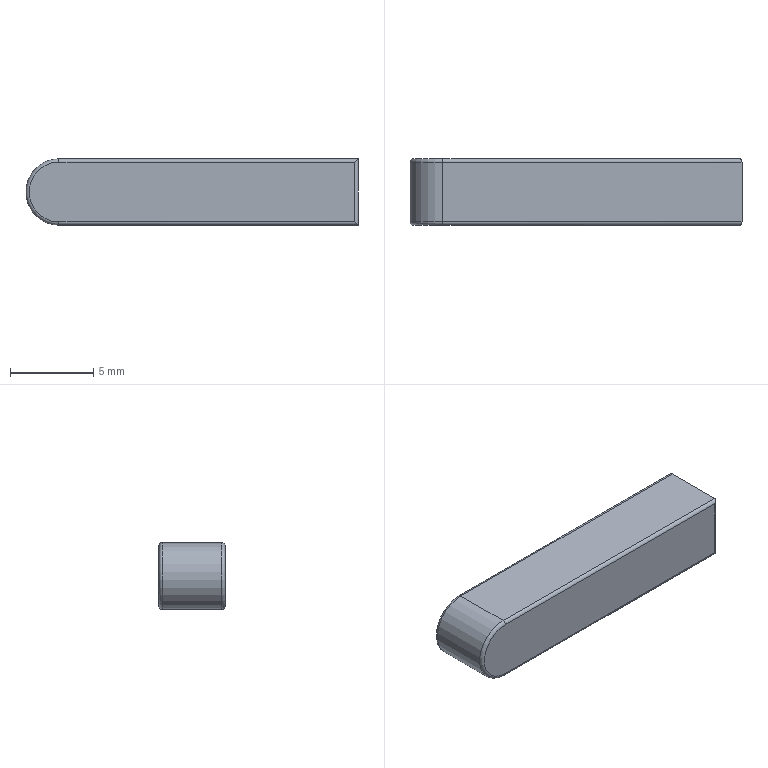Part | STEP file | 1 solid | 14 faces | box 20 x 4 x 4 mm | volume 312.344 mm3 | cylinder 7 | plane 5 | torus 2 | commonest cylinder face diameters 0.4 x6 4 x1
STEP:
#1=CARTESIAN_POINT('',(0.,0.,0.));
#2=DIRECTION('',(0.,0.,1.));
#3=DIRECTION('',(1.,0.,0.));
#4=AXIS2_PLACEMENT_3D('',#1,#2,#3);
#5=CARTESIAN_POINT('',(0.,1.8,-2.));
#6=VERTEX_POINT('',#5);
#7=CARTESIAN_POINT('',(0.,-1.8,-2.));
#8=VERTEX_POINT('',#7);
#9=CARTESIAN_POINT('',(0.,2.,-2.));
#10=DIRECTION('',(0.,-1.,0.));
#11=VECTOR('',#10,1.);
#12=LINE('',#9,#11);
#13=CARTESIAN_POINT('',(0.,2.,0.));
#14=DIRECTION('',(0.,-1.,0.));
#15=DIRECTION('',(0.,0.,-1.));
#16=AXIS2_PLACEMENT_3D('',#13,#14,#15);
#17=CYLINDRICAL_SURFACE('',#16,2.);
#18=CARTESIAN_POINT('',(6.283,0.));
#19=DIRECTION('',(0.,1.));
#20=VECTOR('',#19,1.);
#21=LINE('',#18,#20);
#22=(GEOMETRIC_REPRESENTATION_CONTEXT(2)PARAMETRIC_REPRESENTATION_CONTEXT()REPRESENTATION_CONTEXT('',''));
#23=DEFINITIONAL_REPRESENTATION('',(#21),#22);
#24=PCURVE('',#17,#23);
#25=CARTESIAN_POINT('',(0.,2.,-2.));
#26=DIRECTION('',(0.,0.,1.));
#27=DIRECTION('',(1.,0.,0.));
#28=AXIS2_PLACEMENT_3D('',#25,#26,#27);
#29=PLANE('',#28);
#30=CARTESIAN_POINT('',(0.,0.));
#31=DIRECTION('',(0.,-1.));
#32=VECTOR('',#31,1.);
#33=LINE('',#30,#32);
#34=(GEOMETRIC_REPRESENTATION_CONTEXT(2)PARAMETRIC_REPRESENTATION_CONTEXT()REPRESENTATION_CONTEXT('',''));
#35=DEFINITIONAL_REPRESENTATION('',(#33),#34);
#36=PCURVE('',#29,#35);
#37=SURFACE_CURVE('',#12,(#24,#36),.PCURVE_S1.);
#38=EDGE_CURVE('',#6,#8,#37,.T.);
#39=ORIENTED_EDGE('',*,*,#38,.T.);
#40=CARTESIAN_POINT('',(0.,-1.8,2.));
#41=VERTEX_POINT('',#40);
#42=CARTESIAN_POINT('',(0.,-1.8,0.));
#43=DIRECTION('',(0.,1.,0.));
#44=DIRECTION('',(0.,0.,1.));
#45=AXIS2_PLACEMENT_3D('',#42,#43,#44);
#46=CIRCLE('',#45,2.);
#47=CARTESIAN_POINT('',(9.425,3.8));
#48=DIRECTION('',(-1.,0.));
#49=VECTOR('',#48,1.);
#50=LINE('',#47,#49);
#51=(GEOMETRIC_REPRESENTATION_CONTEXT(2)PARAMETRIC_REPRESENTATION_CONTEXT()REPRESENTATION_CONTEXT('',''));
#52=DEFINITIONAL_REPRESENTATION('',(#50),#51);
#53=PCURVE('',#17,#52);
#54=CARTESIAN_POINT('',(0.,-1.8,0.));
#55=DIRECTION('',(0.,1.,0.));
#56=DIRECTION('',(0.,0.,1.));
#57=AXIS2_PLACEMENT_3D('',#54,#55,#56);
#58=TOROIDAL_SURFACE('',#57,1.8,0.2);
#59=CARTESIAN_POINT('',(0.,6.283));
#60=DIRECTION('',(1.,0.));
#61=VECTOR('',#60,1.);
#62=LINE('',#59,#61);
#63=(GEOMETRIC_REPRESENTATION_CONTEXT(2)PARAMETRIC_REPRESENTATION_CONTEXT()REPRESENTATION_CONTEXT('',''));
#64=DEFINITIONAL_REPRESENTATION('',(#62),#63);
#65=PCURVE('',#58,#64);
#66=SURFACE_CURVE('',#46,(#53,#65),.PCURVE_S1.);
#67=EDGE_CURVE('',#8,#41,#66,.T.);
#68=ORIENTED_EDGE('',*,*,#67,.T.);
#69=CARTESIAN_POINT('',(0.,1.8,2.));
#70=VERTEX_POINT('',#69);
#71=CARTESIAN_POINT('',(0.,2.,2.));
#72=DIRECTION('',(0.,-1.,0.));
#73=VECTOR('',#72,1.);
#74=LINE('',#71,#73);
#75=CARTESIAN_POINT('',(3.142,0.));
#76=DIRECTION('',(0.,1.));
#77=VECTOR('',#76,1.);
#78=LINE('',#75,#77);
#79=(GEOMETRIC_REPRESENTATION_CONTEXT(2)PARAMETRIC_REPRESENTATION_CONTEXT()REPRESENTATION_CONTEXT('',''));
#80=DEFINITIONAL_REPRESENTATION('',(#78),#79);
#81=PCURVE('',#17,#80);
#82=CARTESIAN_POINT('',(0.,2.,2.));
#83=DIRECTION('',(0.,0.,-1.));
#84=DIRECTION('',(-1.,0.,0.));
#85=AXIS2_PLACEMENT_3D('',#82,#83,#84);
#86=PLANE('',#85);
#87=CARTESIAN_POINT('',(0.,0.));
#88=DIRECTION('',(0.,-1.));
#89=VECTOR('',#88,1.);
#90=LINE('',#87,#89);
#91=(GEOMETRIC_REPRESENTATION_CONTEXT(2)PARAMETRIC_REPRESENTATION_CONTEXT()REPRESENTATION_CONTEXT('',''));
#92=DEFINITIONAL_REPRESENTATION('',(#90),#91);
#93=PCURVE('',#86,#92);
#94=SURFACE_CURVE('',#74,(#81,#93),.PCURVE_S1.);
#95=EDGE_CURVE('',#70,#41,#94,.T.);
#96=ORIENTED_EDGE('',*,*,#95,.F.);
#97=CARTESIAN_POINT('',(0.,1.8,0.));
#98=DIRECTION('',(0.,-1.,0.));
#99=DIRECTION('',(0.,0.,1.));
#100=AXIS2_PLACEMENT_3D('',#97,#98,#99);
#101=CIRCLE('',#100,2.);
#102=CARTESIAN_POINT('',(3.142,0.2));
#103=DIRECTION('',(1.,0.));
#104=VECTOR('',#103,1.);
#105=LINE('',#102,#104);
#106=(GEOMETRIC_REPRESENTATION_CONTEXT(2)PARAMETRIC_REPRESENTATION_CONTEXT()REPRESENTATION_CONTEXT('',''));
#107=DEFINITIONAL_REPRESENTATION('',(#105),#106);
#108=PCURVE('',#17,#107);
#109=CARTESIAN_POINT('',(0.,1.8,0.));
#110=DIRECTION('',(0.,1.,0.));
#111=DIRECTION('',(0.,0.,1.));
#112=AXIS2_PLACEMENT_3D('',#109,#110,#111);
#113=TOROIDAL_SURFACE('',#112,1.8,0.2);
#114=CARTESIAN_POINT('',(6.283,0.));
#115=DIRECTION('',(-1.,0.));
#116=VECTOR('',#115,1.);
#117=LINE('',#114,#116);
#118=(GEOMETRIC_REPRESENTATION_CONTEXT(2)PARAMETRIC_REPRESENTATION_CONTEXT()REPRESENTATION_CONTEXT('',''));
#119=DEFINITIONAL_REPRESENTATION('',(#117),#118);
#120=PCURVE('',#113,#119);
#121=SURFACE_CURVE('',#101,(#108,#120),.PCURVE_S1.);
#122=EDGE_CURVE('',#70,#6,#121,.T.);
#123=ORIENTED_EDGE('',*,*,#122,.T.);
#124=EDGE_LOOP('',(#39,#68,#96,#123));
#125=FACE_BOUND('',#124,.T.);
#126=ADVANCED_FACE('',(#125),#17,.T.);
#127=ORIENTED_EDGE('',*,*,#95,.T.);
#128=CARTESIAN_POINT('',(18.,-1.8,2.));
#129=VERTEX_POINT('',#128);
#130=CARTESIAN_POINT('',(0.,-1.8,2.));
#131=DIRECTION('',(1.,0.,0.));
#132=VECTOR('',#131,1.);
#133=LINE('',#130,#132);
#134=CARTESIAN_POINT('',(0.,-3.8));
#135=DIRECTION('',(-1.,0.));
#136=VECTOR('',#135,1.);
#137=LINE('',#134,#136);
#138=(GEOMETRIC_REPRESENTATION_CONTEXT(2)PARAMETRIC_REPRESENTATION_CONTEXT()REPRESENTATION_CONTEXT('',''));
#139=DEFINITIONAL_REPRESENTATION('',(#137),#138);
#140=PCURVE('',#86,#139);
#141=CARTESIAN_POINT('',(0.,-1.8,1.8));
#142=DIRECTION('',(1.,0.,0.));
#143=DIRECTION('',(0.,0.,-1.));
#144=AXIS2_PLACEMENT_3D('',#141,#142,#143);
#145=CYLINDRICAL_SURFACE('',#144,0.2);
#146=CARTESIAN_POINT('',(3.142,0.));
#147=DIRECTION('',(0.,1.));
#148=VECTOR('',#147,1.);
#149=LINE('',#146,#148);
#150=(GEOMETRIC_REPRESENTATION_CONTEXT(2)PARAMETRIC_REPRESENTATION_CONTEXT()REPRESENTATION_CONTEXT('',''));
#151=DEFINITIONAL_REPRESENTATION('',(#149),#150);
#152=PCURVE('',#145,#151);
#153=SURFACE_CURVE('',#133,(#140,#152),.PCURVE_S1.);
#154=EDGE_CURVE('',#41,#129,#153,.T.);
#155=ORIENTED_EDGE('',*,*,#154,.T.);
#156=CARTESIAN_POINT('',(18.,1.8,2.));
#157=VERTEX_POINT('',#156);
#158=CARTESIAN_POINT('',(18.,2.,2.));
#159=DIRECTION('',(0.,-1.,0.));
#160=VECTOR('',#159,1.);
#161=LINE('',#158,#160);
#162=CARTESIAN_POINT('',(-18.,0.));
#163=DIRECTION('',(0.,-1.));
#164=VECTOR('',#163,1.);
#165=LINE('',#162,#164);
#166=(GEOMETRIC_REPRESENTATION_CONTEXT(2)PARAMETRIC_REPRESENTATION_CONTEXT()REPRESENTATION_CONTEXT('',''));
#167=DEFINITIONAL_REPRESENTATION('',(#165),#166);
#168=PCURVE('',#86,#167);
#169=CARTESIAN_POINT('',(18.,-2.,-2.));
#170=DIRECTION('',(-1.,0.,0.));
#171=DIRECTION('',(0.,0.,1.));
#172=AXIS2_PLACEMENT_3D('',#169,#170,#171);
#173=PLANE('',#172);
#174=CARTESIAN_POINT('',(4.,4.));
#175=DIRECTION('',(0.,-1.));
#176=VECTOR('',#175,1.);
#177=LINE('',#174,#176);
#178=(GEOMETRIC_REPRESENTATION_CONTEXT(2)PARAMETRIC_REPRESENTATION_CONTEXT()REPRESENTATION_CONTEXT('',''));
#179=DEFINITIONAL_REPRESENTATION('',(#177),#178);
#180=PCURVE('',#173,#179);
#181=SURFACE_CURVE('',#161,(#168,#180),.PCURVE_S1.);
#182=EDGE_CURVE('',#157,#129,#181,.T.);
#183=ORIENTED_EDGE('',*,*,#182,.F.);
#184=CARTESIAN_POINT('',(0.,1.8,2.));
#185=DIRECTION('',(-1.,0.,0.));
#186=VECTOR('',#185,1.);
#187=LINE('',#184,#186);
#188=CARTESIAN_POINT('',(0.,-0.2));
#189=DIRECTION('',(1.,0.));
#190=VECTOR('',#189,1.);
#191=LINE('',#188,#190);
#192=(GEOMETRIC_REPRESENTATION_CONTEXT(2)PARAMETRIC_REPRESENTATION_CONTEXT()REPRESENTATION_CONTEXT('',''));
#193=DEFINITIONAL_REPRESENTATION('',(#191),#192);
#194=PCURVE('',#86,#193);
#195=CARTESIAN_POINT('',(0.,1.8,1.8));
#196=DIRECTION('',(-1.,0.,0.));
#197=DIRECTION('',(0.,0.,1.));
#198=AXIS2_PLACEMENT_3D('',#195,#196,#197);
#199=CYLINDRICAL_SURFACE('',#198,0.2);
#200=CARTESIAN_POINT('',(0.,0.));
#201=DIRECTION('',(0.,1.));
#202=VECTOR('',#201,1.);
#203=LINE('',#200,#202);
#204=(GEOMETRIC_REPRESENTATION_CONTEXT(2)PARAMETRIC_REPRESENTATION_CONTEXT()REPRESENTATION_CONTEXT('',''));
#205=DEFINITIONAL_REPRESENTATION('',(#203),#204);
#206=PCURVE('',#199,#205);
#207=SURFACE_CURVE('',#187,(#194,#206),.PCURVE_S1.);
#208=EDGE_CURVE('',#157,#70,#207,.T.);
#209=ORIENTED_EDGE('',*,*,#208,.T.);
#210=EDGE_LOOP('',(#127,#155,#183,#209));
#211=FACE_BOUND('',#210,.T.);
#212=ADVANCED_FACE('',(#211),#86,.F.);
#213=CARTESIAN_POINT('',(18.,1.8,-2.));
#214=VERTEX_POINT('',#213);
#215=CARTESIAN_POINT('',(18.,-1.8,-2.));
#216=VERTEX_POINT('',#215);
#217=CARTESIAN_POINT('',(18.,2.,-2.));
#218=DIRECTION('',(0.,-1.,0.));
#219=VECTOR('',#218,1.);
#220=LINE('',#217,#219);
#221=CARTESIAN_POINT('',(18.,0.));
#222=DIRECTION('',(0.,-1.));
#223=VECTOR('',#222,1.);
#224=LINE('',#221,#223);
#225=(GEOMETRIC_REPRESENTATION_CONTEXT(2)PARAMETRIC_REPRESENTATION_CONTEXT()REPRESENTATION_CONTEXT('',''));
#226=DEFINITIONAL_REPRESENTATION('',(#224),#225);
#227=PCURVE('',#29,#226);
#228=CARTESIAN_POINT('',(0.,4.));
#229=DIRECTION('',(0.,-1.));
#230=VECTOR('',#229,1.);
#231=LINE('',#228,#230);
#232=(GEOMETRIC_REPRESENTATION_CONTEXT(2)PARAMETRIC_REPRESENTATION_CONTEXT()REPRESENTATION_CONTEXT('',''));
#233=DEFINITIONAL_REPRESENTATION('',(#231),#232);
#234=PCURVE('',#173,#233);
#235=SURFACE_CURVE('',#220,(#227,#234),.PCURVE_S1.);
#236=EDGE_CURVE('',#214,#216,#235,.T.);
#237=ORIENTED_EDGE('',*,*,#236,.T.);
#238=CARTESIAN_POINT('',(0.,-1.8,-2.));
#239=DIRECTION('',(-1.,0.,0.));
#240=VECTOR('',#239,1.);
#241=LINE('',#238,#240);
#242=CARTESIAN_POINT('',(0.,-3.8));
#243=DIRECTION('',(-1.,0.));
#244=VECTOR('',#243,1.);
#245=LINE('',#242,#244);
#246=(GEOMETRIC_REPRESENTATION_CONTEXT(2)PARAMETRIC_REPRESENTATION_CONTEXT()REPRESENTATION_CONTEXT('',''));
#247=DEFINITIONAL_REPRESENTATION('',(#245),#246);
#248=PCURVE('',#29,#247);
#249=CARTESIAN_POINT('',(0.,-1.8,-1.8));
#250=DIRECTION('',(-1.,0.,0.));
#251=DIRECTION('',(0.,0.,1.));
#252=AXIS2_PLACEMENT_3D('',#249,#250,#251);
#253=CYLINDRICAL_SURFACE('',#252,0.2);
#254=CARTESIAN_POINT('',(3.142,0.));
#255=DIRECTION('',(0.,1.));
#256=VECTOR('',#255,1.);
#257=LINE('',#254,#256);
#258=(GEOMETRIC_REPRESENTATION_CONTEXT(2)PARAMETRIC_REPRESENTATION_CONTEXT()REPRESENTATION_CONTEXT('',''));
#259=DEFINITIONAL_REPRESENTATION('',(#257),#258);
#260=PCURVE('',#253,#259);
#261=SURFACE_CURVE('',#241,(#248,#260),.PCURVE_S1.);
#262=EDGE_CURVE('',#216,#8,#261,.T.);
#263=ORIENTED_EDGE('',*,*,#262,.T.);
#264=ORIENTED_EDGE('',*,*,#38,.F.);
#265=CARTESIAN_POINT('',(18.,1.8,-2.));
#266=DIRECTION('',(1.,0.,0.));
#267=VECTOR('',#266,1.);
#268=LINE('',#265,#267);
#269=CARTESIAN_POINT('',(18.,-0.2));
#270=DIRECTION('',(1.,0.));
#271=VECTOR('',#270,1.);
#272=LINE('',#269,#271);
#273=(GEOMETRIC_REPRESENTATION_CONTEXT(2)PARAMETRIC_REPRESENTATION_CONTEXT()REPRESENTATION_CONTEXT('',''));
#274=DEFINITIONAL_REPRESENTATION('',(#272),#273);
#275=PCURVE('',#29,#274);
#276=CARTESIAN_POINT('',(0.,1.8,-1.8));
#277=DIRECTION('',(1.,0.,0.));
#278=DIRECTION('',(0.,0.,-1.));
#279=AXIS2_PLACEMENT_3D('',#276,#277,#278);
#280=CYLINDRICAL_SURFACE('',#279,0.2);
#281=CARTESIAN_POINT('',(0.,18.));
#282=DIRECTION('',(0.,1.));
#283=VECTOR('',#282,1.);
#284=LINE('',#281,#283);
#285=(GEOMETRIC_REPRESENTATION_CONTEXT(2)PARAMETRIC_REPRESENTATION_CONTEXT()REPRESENTATION_CONTEXT('',''));
#286=DEFINITIONAL_REPRESENTATION('',(#284),#285);
#287=PCURVE('',#280,#286);
#288=SURFACE_CURVE('',#268,(#275,#287),.PCURVE_S1.);
#289=EDGE_CURVE('',#6,#214,#288,.T.);
#290=ORIENTED_EDGE('',*,*,#289,.T.);
#291=EDGE_LOOP('',(#237,#263,#264,#290));
#292=FACE_BOUND('',#291,.T.);
#293=ADVANCED_FACE('',(#292),#29,.F.);
#294=CARTESIAN_POINT('',(0.,2.,-1.8));
#295=VERTEX_POINT('',#294);
#296=CARTESIAN_POINT('',(0.,2.,1.8));
#297=VERTEX_POINT('',#296);
#298=CARTESIAN_POINT('',(0.,2.,0.));
#299=DIRECTION('',(0.,1.,0.));
#300=DIRECTION('',(0.,0.,1.));
#301=AXIS2_PLACEMENT_3D('',#298,#299,#300);
#302=CIRCLE('',#301,1.8);
#303=CARTESIAN_POINT('',(0.,2.,0.));
#304=DIRECTION('',(0.,1.,0.));
#305=DIRECTION('',(0.,0.,1.));
#306=AXIS2_PLACEMENT_3D('',#303,#304,#305);
#307=PLANE('',#306);
#308=CARTESIAN_POINT('',(0.,0.));
#309=DIRECTION('',(1.,0.));
#310=AXIS2_PLACEMENT_2D('',#308,#309);
#311=CIRCLE('',#310,1.8);
#312=(GEOMETRIC_REPRESENTATION_CONTEXT(2)PARAMETRIC_REPRESENTATION_CONTEXT()REPRESENTATION_CONTEXT('',''));
#313=DEFINITIONAL_REPRESENTATION('',(#311),#312);
#314=PCURVE('',#307,#313);
#315=CARTESIAN_POINT('',(0.,1.571));
#316=DIRECTION('',(1.,0.));
#317=VECTOR('',#316,1.);
#318=LINE('',#315,#317);
#319=(GEOMETRIC_REPRESENTATION_CONTEXT(2)PARAMETRIC_REPRESENTATION_CONTEXT()REPRESENTATION_CONTEXT('',''));
#320=DEFINITIONAL_REPRESENTATION('',(#318),#319);
#321=PCURVE('',#113,#320);
#322=SURFACE_CURVE('',#302,(#314,#321),.PCURVE_S1.);
#323=EDGE_CURVE('',#295,#297,#322,.T.);
#324=ORIENTED_EDGE('',*,*,#323,.T.);
#325=CARTESIAN_POINT('',(17.8,2.,1.8));
#326=VERTEX_POINT('',#325);
#327=CARTESIAN_POINT('',(18.,2.,1.8));
#328=DIRECTION('',(1.,0.,0.));
#329=VECTOR('',#328,1.);
#330=LINE('',#327,#329);
#331=CARTESIAN_POINT('',(1.8,18.));
#332=DIRECTION('',(0.,1.));
#333=VECTOR('',#332,1.);
#334=LINE('',#331,#333);
#335=(GEOMETRIC_REPRESENTATION_CONTEXT(2)PARAMETRIC_REPRESENTATION_CONTEXT()REPRESENTATION_CONTEXT('',''));
#336=DEFINITIONAL_REPRESENTATION('',(#334),#335);
#337=PCURVE('',#307,#336);
#338=CARTESIAN_POINT('',(1.571,-18.));
#339=DIRECTION('',(0.,-1.));
#340=VECTOR('',#339,1.);
#341=LINE('',#338,#340);
#342=(GEOMETRIC_REPRESENTATION_CONTEXT(2)PARAMETRIC_REPRESENTATION_CONTEXT()REPRESENTATION_CONTEXT('',''));
#343=DEFINITIONAL_REPRESENTATION('',(#341),#342);
#344=PCURVE('',#199,#343);
#345=SURFACE_CURVE('',#330,(#337,#344),.PCURVE_S1.);
#346=EDGE_CURVE('',#297,#326,#345,.T.);
#347=ORIENTED_EDGE('',*,*,#346,.T.);
#348=CARTESIAN_POINT('',(17.8,2.,-1.8));
#349=VERTEX_POINT('',#348);
#350=CARTESIAN_POINT('',(17.8,2.,-2.));
#351=DIRECTION('',(0.,0.,-1.));
#352=VECTOR('',#351,1.);
#353=LINE('',#350,#352);
#354=CARTESIAN_POINT('',(-2.,17.8));
#355=DIRECTION('',(-1.,0.));
#356=VECTOR('',#355,1.);
#357=LINE('',#354,#356);
#358=(GEOMETRIC_REPRESENTATION_CONTEXT(2)PARAMETRIC_REPRESENTATION_CONTEXT()REPRESENTATION_CONTEXT('',''));
#359=DEFINITIONAL_REPRESENTATION('',(#357),#358);
#360=PCURVE('',#307,#359);
#361=CARTESIAN_POINT('',(17.8,1.8,-2.));
#362=DIRECTION('',(0.,0.,-1.));
#363=DIRECTION('',(-1.,0.,0.));
#364=AXIS2_PLACEMENT_3D('',#361,#362,#363);
#365=CYLINDRICAL_SURFACE('',#364,0.2);
#366=CARTESIAN_POINT('',(1.571,0.));
#367=DIRECTION('',(0.,1.));
#368=VECTOR('',#367,1.);
#369=LINE('',#366,#368);
#370=(GEOMETRIC_REPRESENTATION_CONTEXT(2)PARAMETRIC_REPRESENTATION_CONTEXT()REPRESENTATION_CONTEXT('',''));
#371=DEFINITIONAL_REPRESENTATION('',(#369),#370);
#372=PCURVE('',#365,#371);
#373=SURFACE_CURVE('',#353,(#360,#372),.PCURVE_S1.);
#374=EDGE_CURVE('',#326,#349,#373,.T.);
#375=ORIENTED_EDGE('',*,*,#374,.T.);
#376=CARTESIAN_POINT('',(0.,2.,-1.8));
#377=DIRECTION('',(-1.,0.,0.));
#378=VECTOR('',#377,1.);
#379=LINE('',#376,#378);
#380=CARTESIAN_POINT('',(-1.8,0.));
#381=DIRECTION('',(0.,-1.));
#382=VECTOR('',#381,1.);
#383=LINE('',#380,#382);
#384=(GEOMETRIC_REPRESENTATION_CONTEXT(2)PARAMETRIC_REPRESENTATION_CONTEXT()REPRESENTATION_CONTEXT('',''));
#385=DEFINITIONAL_REPRESENTATION('',(#383),#384);
#386=PCURVE('',#307,#385);
#387=CARTESIAN_POINT('',(1.571,0.));
#388=DIRECTION('',(0.,-1.));
#389=VECTOR('',#388,1.);
#390=LINE('',#387,#389);
#391=(GEOMETRIC_REPRESENTATION_CONTEXT(2)PARAMETRIC_REPRESENTATION_CONTEXT()REPRESENTATION_CONTEXT('',''));
#392=DEFINITIONAL_REPRESENTATION('',(#390),#391);
#393=PCURVE('',#280,#392);
#394=SURFACE_CURVE('',#379,(#386,#393),.PCURVE_S1.);
#395=EDGE_CURVE('',#349,#295,#394,.T.);
#396=ORIENTED_EDGE('',*,*,#395,.T.);
#397=EDGE_LOOP('',(#324,#347,#375,#396));
#398=FACE_BOUND('',#397,.T.);
#399=ADVANCED_FACE('',(#398),#307,.T.);
#400=CARTESIAN_POINT('',(17.8,-2.,1.8));
#401=VERTEX_POINT('',#400);
#402=CARTESIAN_POINT('',(0.,-2.,1.8));
#403=VERTEX_POINT('',#402);
#404=CARTESIAN_POINT('',(0.,-2.,1.8));
#405=DIRECTION('',(-1.,0.,0.));
#406=VECTOR('',#405,1.);
#407=LINE('',#404,#406);
#408=CARTESIAN_POINT('',(0.,-2.,0.));
#409=DIRECTION('',(0.,1.,0.));
#410=DIRECTION('',(0.,0.,1.));
#411=AXIS2_PLACEMENT_3D('',#408,#409,#410);
#412=PLANE('',#411);
#413=CARTESIAN_POINT('',(1.8,0.));
#414=DIRECTION('',(0.,-1.));
#415=VECTOR('',#414,1.);
#416=LINE('',#413,#415);
#417=(GEOMETRIC_REPRESENTATION_CONTEXT(2)PARAMETRIC_REPRESENTATION_CONTEXT()REPRESENTATION_CONTEXT('',''));
#418=DEFINITIONAL_REPRESENTATION('',(#416),#417);
#419=PCURVE('',#412,#418);
#420=CARTESIAN_POINT('',(4.712,0.));
#421=DIRECTION('',(0.,-1.));
#422=VECTOR('',#421,1.);
#423=LINE('',#420,#422);
#424=(GEOMETRIC_REPRESENTATION_CONTEXT(2)PARAMETRIC_REPRESENTATION_CONTEXT()REPRESENTATION_CONTEXT('',''));
#425=DEFINITIONAL_REPRESENTATION('',(#423),#424);
#426=PCURVE('',#145,#425);
#427=SURFACE_CURVE('',#407,(#419,#426),.PCURVE_S1.);
#428=EDGE_CURVE('',#401,#403,#427,.T.);
#429=ORIENTED_EDGE('',*,*,#428,.T.);
#430=CARTESIAN_POINT('',(0.,-2.,-1.8));
#431=VERTEX_POINT('',#430);
#432=CARTESIAN_POINT('',(0.,-2.,0.));
#433=DIRECTION('',(0.,-1.,0.));
#434=DIRECTION('',(0.,0.,1.));
#435=AXIS2_PLACEMENT_3D('',#432,#433,#434);
#436=CIRCLE('',#435,1.8);
#437=CARTESIAN_POINT('',(1.8,0.));
#438=CARTESIAN_POINT('',(1.8,-3.118));
#439=CARTESIAN_POINT('',(-0.9,-1.559));
#440=CARTESIAN_POINT('',(-3.6,0.));
#441=CARTESIAN_POINT('',(-0.9,1.559));
#442=CARTESIAN_POINT('',(1.8,3.118));
#443=CARTESIAN_POINT('',(1.8,0.));
#444=(BOUNDED_CURVE()B_SPLINE_CURVE(2,(#437,#438,#439,#440,#441,#442,#443),.UNSPECIFIED.,.T.,.F.)B_SPLINE_CURVE_WITH_KNOTS((1,2,2,2,2,1),(-2.094,0.,2.094,4.189,6.283,8.378),.UNSPECIFIED.)CURVE()GEOMETRIC_REPRESENTATION_ITEM()RATIONAL_B_SPLINE_CURVE((1.,0.5,1.,0.5,1.,0.5,1.))REPRESENTATION_ITEM(''));
#445=(GEOMETRIC_REPRESENTATION_CONTEXT(2)PARAMETRIC_REPRESENTATION_CONTEXT()REPRESENTATION_CONTEXT('',''));
#446=DEFINITIONAL_REPRESENTATION('',(#444),#445);
#447=PCURVE('',#412,#446);
#448=CARTESIAN_POINT('',(6.283,4.712));
#449=DIRECTION('',(-1.,0.));
#450=VECTOR('',#449,1.);
#451=LINE('',#448,#450);
#452=(GEOMETRIC_REPRESENTATION_CONTEXT(2)PARAMETRIC_REPRESENTATION_CONTEXT()REPRESENTATION_CONTEXT('',''));
#453=DEFINITIONAL_REPRESENTATION('',(#451),#452);
#454=PCURVE('',#58,#453);
#455=SURFACE_CURVE('',#436,(#447,#454),.PCURVE_S1.);
#456=EDGE_CURVE('',#403,#431,#455,.T.);
#457=ORIENTED_EDGE('',*,*,#456,.T.);
#458=CARTESIAN_POINT('',(17.8,-2.,-1.8));
#459=VERTEX_POINT('',#458);
#460=CARTESIAN_POINT('',(0.,-2.,-1.8));
#461=DIRECTION('',(1.,0.,0.));
#462=VECTOR('',#461,1.);
#463=LINE('',#460,#462);
#464=CARTESIAN_POINT('',(-1.8,0.));
#465=DIRECTION('',(0.,1.));
#466=VECTOR('',#465,1.);
#467=LINE('',#464,#466);
#468=(GEOMETRIC_REPRESENTATION_CONTEXT(2)PARAMETRIC_REPRESENTATION_CONTEXT()REPRESENTATION_CONTEXT('',''));
#469=DEFINITIONAL_REPRESENTATION('',(#467),#468);
#470=PCURVE('',#412,#469);
#471=CARTESIAN_POINT('',(4.712,0.));
#472=DIRECTION('',(0.,-1.));
#473=VECTOR('',#472,1.);
#474=LINE('',#471,#473);
#475=(GEOMETRIC_REPRESENTATION_CONTEXT(2)PARAMETRIC_REPRESENTATION_CONTEXT()REPRESENTATION_CONTEXT('',''));
#476=DEFINITIONAL_REPRESENTATION('',(#474),#475);
#477=PCURVE('',#253,#476);
#478=SURFACE_CURVE('',#463,(#470,#477),.PCURVE_S1.);
#479=EDGE_CURVE('',#431,#459,#478,.T.);
#480=ORIENTED_EDGE('',*,*,#479,.T.);
#481=CARTESIAN_POINT('',(17.8,-2.,0.));
#482=DIRECTION('',(0.,0.,1.));
#483=VECTOR('',#482,1.);
#484=LINE('',#481,#483);
#485=CARTESIAN_POINT('',(0.,17.8));
#486=DIRECTION('',(1.,0.));
#487=VECTOR('',#486,1.);
#488=LINE('',#485,#487);
#489=(GEOMETRIC_REPRESENTATION_CONTEXT(2)PARAMETRIC_REPRESENTATION_CONTEXT()REPRESENTATION_CONTEXT('',''));
#490=DEFINITIONAL_REPRESENTATION('',(#488),#489);
#491=PCURVE('',#412,#490);
#492=CARTESIAN_POINT('',(17.8,-1.8,0.));
#493=DIRECTION('',(0.,0.,1.));
#494=DIRECTION('',(1.,0.,0.));
#495=AXIS2_PLACEMENT_3D('',#492,#493,#494);
#496=CYLINDRICAL_SURFACE('',#495,0.2);
#497=CARTESIAN_POINT('',(4.712,0.));
#498=DIRECTION('',(0.,1.));
#499=VECTOR('',#498,1.);
#500=LINE('',#497,#499);
#501=(GEOMETRIC_REPRESENTATION_CONTEXT(2)PARAMETRIC_REPRESENTATION_CONTEXT()REPRESENTATION_CONTEXT('',''));
#502=DEFINITIONAL_REPRESENTATION('',(#500),#501);
#503=PCURVE('',#496,#502);
#504=SURFACE_CURVE('',#484,(#491,#503),.PCURVE_S1.);
#505=EDGE_CURVE('',#459,#401,#504,.T.);
#506=ORIENTED_EDGE('',*,*,#505,.T.);
#507=EDGE_LOOP('',(#429,#457,#480,#506));
#508=FACE_BOUND('',#507,.T.);
#509=ADVANCED_FACE('',(#508),#412,.F.);
#510=ORIENTED_EDGE('',*,*,#182,.T.);
#511=CARTESIAN_POINT('',(18.,-1.8,-2.));
#512=DIRECTION('',(0.,0.,-1.));
#513=VECTOR('',#512,1.);
#514=LINE('',#511,#513);
#515=CARTESIAN_POINT('',(0.,0.2));
#516=DIRECTION('',(-1.,0.));
#517=VECTOR('',#516,1.);
#518=LINE('',#515,#517);
#519=(GEOMETRIC_REPRESENTATION_CONTEXT(2)PARAMETRIC_REPRESENTATION_CONTEXT()REPRESENTATION_CONTEXT('',''));
#520=DEFINITIONAL_REPRESENTATION('',(#518),#519);
#521=PCURVE('',#173,#520);
#522=CARTESIAN_POINT('',(6.283,-2.));
#523=DIRECTION('',(0.,-1.));
#524=VECTOR('',#523,1.);
#525=LINE('',#522,#524);
#526=(GEOMETRIC_REPRESENTATION_CONTEXT(2)PARAMETRIC_REPRESENTATION_CONTEXT()REPRESENTATION_CONTEXT('',''));
#527=DEFINITIONAL_REPRESENTATION('',(#525),#526);
#528=PCURVE('',#496,#527);
#529=SURFACE_CURVE('',#514,(#521,#528),.PCURVE_S1.);
#530=EDGE_CURVE('',#129,#216,#529,.T.);
#531=ORIENTED_EDGE('',*,*,#530,.T.);
#532=ORIENTED_EDGE('',*,*,#236,.F.);
#533=CARTESIAN_POINT('',(18.,1.8,2.));
#534=DIRECTION('',(0.,0.,1.));
#535=VECTOR('',#534,1.);
#536=LINE('',#533,#535);
#537=CARTESIAN_POINT('',(4.,3.8));
#538=DIRECTION('',(1.,0.));
#539=VECTOR('',#538,1.);
#540=LINE('',#537,#539);
#541=(GEOMETRIC_REPRESENTATION_CONTEXT(2)PARAMETRIC_REPRESENTATION_CONTEXT()REPRESENTATION_CONTEXT('',''));
#542=DEFINITIONAL_REPRESENTATION('',(#540),#541);
#543=PCURVE('',#173,#542);
#544=CARTESIAN_POINT('',(3.142,-4.));
#545=DIRECTION('',(0.,-1.));
#546=VECTOR('',#545,1.);
#547=LINE('',#544,#546);
#548=(GEOMETRIC_REPRESENTATION_CONTEXT(2)PARAMETRIC_REPRESENTATION_CONTEXT()REPRESENTATION_CONTEXT('',''));
#549=DEFINITIONAL_REPRESENTATION('',(#547),#548);
#550=PCURVE('',#365,#549);
#551=SURFACE_CURVE('',#536,(#543,#550),.PCURVE_S1.);
#552=EDGE_CURVE('',#214,#157,#551,.T.);
#553=ORIENTED_EDGE('',*,*,#552,.T.);
#554=EDGE_LOOP('',(#510,#531,#532,#553));
#555=FACE_BOUND('',#554,.T.);
#556=ADVANCED_FACE('',(#555),#173,.F.);
#557=CARTESIAN_POINT('',(17.8,-2.,1.8));
#558=CARTESIAN_POINT('',(17.917,-2.,1.917));
#559=CARTESIAN_POINT('',(18.,-1.917,2.));
#560=CARTESIAN_POINT('',(18.,-1.8,2.));
#561=(BOUNDED_CURVE()B_SPLINE_CURVE(3,(#557,#558,#559,#560),.UNSPECIFIED.,.F.,.F.)B_SPLINE_CURVE_WITH_KNOTS((4,4),(4.712,6.283),.PIECEWISE_BEZIER_KNOTS.)CURVE()GEOMETRIC_REPRESENTATION_ITEM()RATIONAL_B_SPLINE_CURVE((1.,0.8047,0.8047,1.))REPRESENTATION_ITEM(''));
#562=CARTESIAN_POINT('',(4.712,1.8));
#563=CARTESIAN_POINT('',(4.734,1.804));
#564=CARTESIAN_POINT('',(4.777,1.813));
#565=CARTESIAN_POINT('',(4.844,1.826));
#566=CARTESIAN_POINT('',(4.912,1.84));
#567=CARTESIAN_POINT('',(4.982,1.853));
#568=CARTESIAN_POINT('',(5.053,1.867));
#569=CARTESIAN_POINT('',(5.125,1.88));
#570=CARTESIAN_POINT('',(5.199,1.894));
#571=CARTESIAN_POINT('',(5.273,1.906));
#572=CARTESIAN_POINT('',(5.347,1.919));
#573=CARTESIAN_POINT('',(5.422,1.931));
#574=CARTESIAN_POINT('',(5.498,1.942));
#575=CARTESIAN_POINT('',(5.573,1.952));
#576=CARTESIAN_POINT('',(5.648,1.961));
#577=CARTESIAN_POINT('',(5.723,1.97));
#578=CARTESIAN_POINT('',(5.797,1.977));
#579=CARTESIAN_POINT('',(5.87,1.983));
#580=CARTESIAN_POINT('',(5.942,1.989));
#581=CARTESIAN_POINT('',(6.013,1.993));
#582=CARTESIAN_POINT('',(6.083,1.996));
#583=CARTESIAN_POINT('',(6.152,1.998));
#584=CARTESIAN_POINT('',(6.218,2.));
#585=CARTESIAN_POINT('',(6.262,2.));
#586=CARTESIAN_POINT('',(6.283,2.));
#587=B_SPLINE_CURVE_WITH_KNOTS('',3,(#562,#563,#564,#565,#566,#567,#568,#569,#570,#571,#572,#573,#574,#575,#576,#577,#578,#579,#580,#581,#582,#583,#584,#585,#586),.UNSPECIFIED.,.F.,.F.,(4,1,1,1,1,1,1,1,1,1,1,1,1,1,1,1,1,1,1,1,1,1,4),(4.712,4.784,4.855,4.927,4.998,5.069,5.141,5.212,5.284,5.355,5.426,5.498,5.569,5.641,5.712,5.783,5.855,5.926,5.998,6.069,6.14,6.212,6.283),.QUASI_UNIFORM_KNOTS.);
#588=(GEOMETRIC_REPRESENTATION_CONTEXT(2)PARAMETRIC_REPRESENTATION_CONTEXT()REPRESENTATION_CONTEXT('',''));
#589=DEFINITIONAL_REPRESENTATION('',(#587),#588);
#590=PCURVE('',#496,#589);
#591=CARTESIAN_POINT('',(4.712,17.8));
#592=CARTESIAN_POINT('',(4.691,17.804));
#593=CARTESIAN_POINT('',(4.648,17.813));
#594=CARTESIAN_POINT('',(4.581,17.826));
#595=CARTESIAN_POINT('',(4.512,17.84));
#596=CARTESIAN_POINT('',(4.443,17.853));
#597=CARTESIAN_POINT('',(4.372,17.867));
#598=CARTESIAN_POINT('',(4.299,17.88));
#599=CARTESIAN_POINT('',(4.226,17.894));
#600=CARTESIAN_POINT('',(4.152,17.906));
#601=CARTESIAN_POINT('',(4.077,17.919));
#602=CARTESIAN_POINT('',(4.002,17.931));
#603=CARTESIAN_POINT('',(3.927,17.942));
#604=CARTESIAN_POINT('',(3.852,17.952));
#605=CARTESIAN_POINT('',(3.777,17.961));
#606=CARTESIAN_POINT('',(3.702,17.97));
#607=CARTESIAN_POINT('',(3.628,17.977));
#608=CARTESIAN_POINT('',(3.555,17.983));
#609=CARTESIAN_POINT('',(3.482,17.989));
#610=CARTESIAN_POINT('',(3.411,17.993));
#611=CARTESIAN_POINT('',(3.342,17.996));
#612=CARTESIAN_POINT('',(3.273,17.998));
#613=CARTESIAN_POINT('',(3.206,18.));
#614=CARTESIAN_POINT('',(3.163,18.));
#615=CARTESIAN_POINT('',(3.142,18.));
#616=B_SPLINE_CURVE_WITH_KNOTS('',3,(#591,#592,#593,#594,#595,#596,#597,#598,#599,#600,#601,#602,#603,#604,#605,#606,#607,#608,#609,#610,#611,#612,#613,#614,#615),.UNSPECIFIED.,.F.,.F.,(4,1,1,1,1,1,1,1,1,1,1,1,1,1,1,1,1,1,1,1,1,1,4),(4.712,4.784,4.855,4.927,4.998,5.069,5.141,5.212,5.284,5.355,5.426,5.498,5.569,5.641,5.712,5.783,5.855,5.926,5.998,6.069,6.14,6.212,6.283),.QUASI_UNIFORM_KNOTS.);
#617=(GEOMETRIC_REPRESENTATION_CONTEXT(2)PARAMETRIC_REPRESENTATION_CONTEXT()REPRESENTATION_CONTEXT('',''));
#618=DEFINITIONAL_REPRESENTATION('',(#616),#617);
#619=PCURVE('',#145,#618);
#620=SURFACE_CURVE('',#561,(#590,#619),.PCURVE_S1.);
#621=EDGE_CURVE('',#401,#129,#620,.T.);
#622=ORIENTED_EDGE('',*,*,#621,.F.);
#623=ORIENTED_EDGE('',*,*,#505,.F.);
#624=CARTESIAN_POINT('',(18.,-1.8,-2.));
#625=CARTESIAN_POINT('',(18.,-1.917,-2.));
#626=CARTESIAN_POINT('',(17.917,-2.,-1.917));
#627=CARTESIAN_POINT('',(17.8,-2.,-1.8));
#628=(BOUNDED_CURVE()B_SPLINE_CURVE(3,(#624,#625,#626,#627),.UNSPECIFIED.,.F.,.F.)B_SPLINE_CURVE_WITH_KNOTS((4,4),(3.142,4.712),.PIECEWISE_BEZIER_KNOTS.)CURVE()GEOMETRIC_REPRESENTATION_ITEM()RATIONAL_B_SPLINE_CURVE((1.,0.8047,0.8047,1.))REPRESENTATION_ITEM(''));
#629=CARTESIAN_POINT('',(6.283,-2.));
#630=CARTESIAN_POINT('',(6.262,-2.));
#631=CARTESIAN_POINT('',(6.218,-2.));
#632=CARTESIAN_POINT('',(6.152,-1.998));
#633=CARTESIAN_POINT('',(6.083,-1.996));
#634=CARTESIAN_POINT('',(6.013,-1.993));
#635=CARTESIAN_POINT('',(5.942,-1.989));
#636=CARTESIAN_POINT('',(5.87,-1.983));
#637=CARTESIAN_POINT('',(5.797,-1.977));
#638=CARTESIAN_POINT('',(5.723,-1.97));
#639=CARTESIAN_POINT('',(5.648,-1.961));
#640=CARTESIAN_POINT('',(5.573,-1.952));
#641=CARTESIAN_POINT('',(5.498,-1.942));
#642=CARTESIAN_POINT('',(5.422,-1.931));
#643=CARTESIAN_POINT('',(5.347,-1.919));
#644=CARTESIAN_POINT('',(5.273,-1.906));
#645=CARTESIAN_POINT('',(5.199,-1.894));
#646=CARTESIAN_POINT('',(5.125,-1.88));
#647=CARTESIAN_POINT('',(5.053,-1.867));
#648=CARTESIAN_POINT('',(4.982,-1.853));
#649=CARTESIAN_POINT('',(4.912,-1.84));
#650=CARTESIAN_POINT('',(4.844,-1.826));
#651=CARTESIAN_POINT('',(4.777,-1.813));
#652=CARTESIAN_POINT('',(4.734,-1.804));
#653=CARTESIAN_POINT('',(4.712,-1.8));
#654=B_SPLINE_CURVE_WITH_KNOTS('',3,(#629,#630,#631,#632,#633,#634,#635,#636,#637,#638,#639,#640,#641,#642,#643,#644,#645,#646,#647,#648,#649,#650,#651,#652,#653),.UNSPECIFIED.,.F.,.F.,(4,1,1,1,1,1,1,1,1,1,1,1,1,1,1,1,1,1,1,1,1,1,4),(3.142,3.213,3.284,3.356,3.427,3.499,3.57,3.641,3.713,3.784,3.856,3.927,3.998,4.07,4.141,4.213,4.284,4.355,4.427,4.498,4.57,4.641,4.712),.QUASI_UNIFORM_KNOTS.);
#655=(GEOMETRIC_REPRESENTATION_CONTEXT(2)PARAMETRIC_REPRESENTATION_CONTEXT()REPRESENTATION_CONTEXT('',''));
#656=DEFINITIONAL_REPRESENTATION('',(#654),#655);
#657=PCURVE('',#496,#656);
#658=CARTESIAN_POINT('',(3.142,-18.));
#659=CARTESIAN_POINT('',(3.163,-18.));
#660=CARTESIAN_POINT('',(3.206,-18.));
#661=CARTESIAN_POINT('',(3.273,-17.998));
#662=CARTESIAN_POINT('',(3.342,-17.996));
#663=CARTESIAN_POINT('',(3.411,-17.993));
#664=CARTESIAN_POINT('',(3.482,-17.989));
#665=CARTESIAN_POINT('',(3.555,-17.983));
#666=CARTESIAN_POINT('',(3.628,-17.977));
#667=CARTESIAN_POINT('',(3.702,-17.97));
#668=CARTESIAN_POINT('',(3.777,-17.961));
#669=CARTESIAN_POINT('',(3.852,-17.952));
#670=CARTESIAN_POINT('',(3.927,-17.942));
#671=CARTESIAN_POINT('',(4.002,-17.931));
#672=CARTESIAN_POINT('',(4.077,-17.919));
#673=CARTESIAN_POINT('',(4.152,-17.906));
#674=CARTESIAN_POINT('',(4.226,-17.894));
#675=CARTESIAN_POINT('',(4.299,-17.88));
#676=CARTESIAN_POINT('',(4.372,-17.867));
#677=CARTESIAN_POINT('',(4.443,-17.853));
#678=CARTESIAN_POINT('',(4.512,-17.84));
#679=CARTESIAN_POINT('',(4.581,-17.826));
#680=CARTESIAN_POINT('',(4.648,-17.813));
#681=CARTESIAN_POINT('',(4.691,-17.804));
#682=CARTESIAN_POINT('',(4.712,-17.8));
#683=B_SPLINE_CURVE_WITH_KNOTS('',3,(#658,#659,#660,#661,#662,#663,#664,#665,#666,#667,#668,#669,#670,#671,#672,#673,#674,#675,#676,#677,#678,#679,#680,#681,#682),.UNSPECIFIED.,.F.,.F.,(4,1,1,1,1,1,1,1,1,1,1,1,1,1,1,1,1,1,1,1,1,1,4),(3.142,3.213,3.284,3.356,3.427,3.499,3.57,3.641,3.713,3.784,3.856,3.927,3.998,4.07,4.141,4.213,4.284,4.355,4.427,4.498,4.57,4.641,4.712),.QUASI_UNIFORM_KNOTS.);
#684=(GEOMETRIC_REPRESENTATION_CONTEXT(2)PARAMETRIC_REPRESENTATION_CONTEXT()REPRESENTATION_CONTEXT('',''));
#685=DEFINITIONAL_REPRESENTATION('',(#683),#684);
#686=PCURVE('',#253,#685);
#687=SURFACE_CURVE('',#628,(#657,#686),.PCURVE_S1.);
#688=EDGE_CURVE('',#216,#459,#687,.T.);
#689=ORIENTED_EDGE('',*,*,#688,.F.);
#690=ORIENTED_EDGE('',*,*,#530,.F.);
#691=EDGE_LOOP('',(#622,#623,#689,#690));
#692=FACE_BOUND('',#691,.T.);
#693=ADVANCED_FACE('',(#692),#496,.T.);
#694=ORIENTED_EDGE('',*,*,#688,.T.);
#695=ORIENTED_EDGE('',*,*,#479,.F.);
#696=CARTESIAN_POINT('',(0.,-1.8,-1.8));
#697=DIRECTION('',(-1.,0.,0.));
#698=DIRECTION('',(0.,0.,1.));
#699=AXIS2_PLACEMENT_3D('',#696,#697,#698);
#700=CIRCLE('',#699,0.2);
#701=CARTESIAN_POINT('',(0.,0.));
#702=DIRECTION('',(1.,0.));
#703=VECTOR('',#702,1.);
#704=LINE('',#701,#703);
#705=(GEOMETRIC_REPRESENTATION_CONTEXT(2)PARAMETRIC_REPRESENTATION_CONTEXT()REPRESENTATION_CONTEXT('',''));
#706=DEFINITIONAL_REPRESENTATION('',(#704),#705);
#707=PCURVE('',#253,#706);
#708=CARTESIAN_POINT('',(3.142,9.425));
#709=DIRECTION('',(0.,-1.));
#710=VECTOR('',#709,1.);
#711=LINE('',#708,#710);
#712=(GEOMETRIC_REPRESENTATION_CONTEXT(2)PARAMETRIC_REPRESENTATION_CONTEXT()REPRESENTATION_CONTEXT('',''));
#713=DEFINITIONAL_REPRESENTATION('',(#711),#712);
#714=PCURVE('',#58,#713);
#715=SURFACE_CURVE('',#700,(#707,#714),.PCURVE_S1.);
#716=EDGE_CURVE('',#8,#431,#715,.T.);
#717=ORIENTED_EDGE('',*,*,#716,.F.);
#718=ORIENTED_EDGE('',*,*,#262,.F.);
#719=EDGE_LOOP('',(#694,#695,#717,#718));
#720=FACE_BOUND('',#719,.T.);
#721=ADVANCED_FACE('',(#720),#253,.T.);
#722=ORIENTED_EDGE('',*,*,#621,.T.);
#723=ORIENTED_EDGE('',*,*,#154,.F.);
#724=CARTESIAN_POINT('',(0.,-1.8,1.8));
#725=DIRECTION('',(-1.,0.,0.));
#726=DIRECTION('',(0.,0.,1.));
#727=AXIS2_PLACEMENT_3D('',#724,#725,#726);
#728=CIRCLE('',#727,0.2);
#729=CARTESIAN_POINT('',(9.425,0.));
#730=DIRECTION('',(-1.,0.));
#731=VECTOR('',#730,1.);
#732=LINE('',#729,#731);
#733=(GEOMETRIC_REPRESENTATION_CONTEXT(2)PARAMETRIC_REPRESENTATION_CONTEXT()REPRESENTATION_CONTEXT('',''));
#734=DEFINITIONAL_REPRESENTATION('',(#732),#733);
#735=PCURVE('',#145,#734);
#736=CARTESIAN_POINT('',(6.283,0.));
#737=DIRECTION('',(0.,1.));
#738=VECTOR('',#737,1.);
#739=LINE('',#736,#738);
#740=(GEOMETRIC_REPRESENTATION_CONTEXT(2)PARAMETRIC_REPRESENTATION_CONTEXT()REPRESENTATION_CONTEXT('',''));
#741=DEFINITIONAL_REPRESENTATION('',(#739),#740);
#742=PCURVE('',#58,#741);
#743=SURFACE_CURVE('',#728,(#735,#742),.PCURVE_S1.);
#744=EDGE_CURVE('',#403,#41,#743,.T.);
#745=ORIENTED_EDGE('',*,*,#744,.F.);
#746=ORIENTED_EDGE('',*,*,#428,.F.);
#747=EDGE_LOOP('',(#722,#723,#745,#746));
#748=FACE_BOUND('',#747,.T.);
#749=ADVANCED_FACE('',(#748),#145,.T.);
#750=ORIENTED_EDGE('',*,*,#716,.T.);
#751=ORIENTED_EDGE('',*,*,#456,.F.);
#752=ORIENTED_EDGE('',*,*,#744,.T.);
#753=ORIENTED_EDGE('',*,*,#67,.F.);
#754=EDGE_LOOP('',(#750,#751,#752,#753));
#755=FACE_BOUND('',#754,.T.);
#756=ADVANCED_FACE('',(#755),#58,.T.);
#757=CARTESIAN_POINT('',(18.,1.8,-2.));
#758=CARTESIAN_POINT('',(18.,1.917,-2.));
#759=CARTESIAN_POINT('',(17.917,2.,-1.917));
#760=CARTESIAN_POINT('',(17.8,2.,-1.8));
#761=(BOUNDED_CURVE()B_SPLINE_CURVE(3,(#757,#758,#759,#760),.UNSPECIFIED.,.F.,.F.)B_SPLINE_CURVE_WITH_KNOTS((4,4),(0.,1.571),.PIECEWISE_BEZIER_KNOTS.)CURVE()GEOMETRIC_REPRESENTATION_ITEM()RATIONAL_B_SPLINE_CURVE((1.,0.8047,0.8047,1.))REPRESENTATION_ITEM(''));
#762=CARTESIAN_POINT('',(0.,18.));
#763=CARTESIAN_POINT('',(0.02143,18.));
#764=CARTESIAN_POINT('',(0.06485,18.));
#765=CARTESIAN_POINT('',(0.1316,17.998));
#766=CARTESIAN_POINT('',(0.2,17.996));
#767=CARTESIAN_POINT('',(0.2697,17.993));
#768=CARTESIAN_POINT('',(0.3408,17.989));
#769=CARTESIAN_POINT('',(0.413,17.983));
#770=CARTESIAN_POINT('',(0.4863,17.977));
#771=CARTESIAN_POINT('',(0.5603,17.97));
#772=CARTESIAN_POINT('',(0.635,17.961));
#773=CARTESIAN_POINT('',(0.7101,17.952));
#774=CARTESIAN_POINT('',(0.7854,17.942));
#775=CARTESIAN_POINT('',(0.8607,17.931));
#776=CARTESIAN_POINT('',(0.9358,17.919));
#777=CARTESIAN_POINT('',(1.01,17.906));
#778=CARTESIAN_POINT('',(1.085,17.894));
#779=CARTESIAN_POINT('',(1.158,17.88));
#780=CARTESIAN_POINT('',(1.23,17.867));
#781=CARTESIAN_POINT('',(1.301,17.853));
#782=CARTESIAN_POINT('',(1.371,17.84));
#783=CARTESIAN_POINT('',(1.439,17.826));
#784=CARTESIAN_POINT('',(1.506,17.813));
#785=CARTESIAN_POINT('',(1.549,17.804));
#786=CARTESIAN_POINT('',(1.571,17.8));
#787=B_SPLINE_CURVE_WITH_KNOTS('',3,(#762,#763,#764,#765,#766,#767,#768,#769,#770,#771,#772,#773,#774,#775,#776,#777,#778,#779,#780,#781,#782,#783,#784,#785,#786),.UNSPECIFIED.,.F.,.F.,(4,1,1,1,1,1,1,1,1,1,1,1,1,1,1,1,1,1,1,1,1,1,4),(0.,0.0714,0.1428,0.2142,0.2856,0.357,0.4284,0.4998,0.5712,0.6426,0.714,0.7854,0.8568,0.9282,0.9996,1.071,1.142,1.214,1.285,1.357,1.428,1.499,1.571),.QUASI_UNIFORM_KNOTS.);
#788=(GEOMETRIC_REPRESENTATION_CONTEXT(2)PARAMETRIC_REPRESENTATION_CONTEXT()REPRESENTATION_CONTEXT('',''));
#789=DEFINITIONAL_REPRESENTATION('',(#787),#788);
#790=PCURVE('',#280,#789);
#791=CARTESIAN_POINT('',(3.142,0.));
#792=CARTESIAN_POINT('',(3.12,0.000000649));
#793=CARTESIAN_POINT('',(3.077,-0.0002759));
#794=CARTESIAN_POINT('',(3.01,-0.001579));
#795=CARTESIAN_POINT('',(2.942,-0.003829));
#796=CARTESIAN_POINT('',(2.872,-0.007072));
#797=CARTESIAN_POINT('',(2.801,-0.01134));
#798=CARTESIAN_POINT('',(2.729,-0.01666));
#799=CARTESIAN_POINT('',(2.655,-0.02302));
#800=CARTESIAN_POINT('',(2.581,-0.03043));
#801=CARTESIAN_POINT('',(2.507,-0.03883));
#802=CARTESIAN_POINT('',(2.432,-0.0482));
#803=CARTESIAN_POINT('',(2.356,-0.05844));
#804=CARTESIAN_POINT('',(2.281,-0.0695));
#805=CARTESIAN_POINT('',(2.206,-0.08126));
#806=CARTESIAN_POINT('',(2.131,-0.09361));
#807=CARTESIAN_POINT('',(2.057,-0.1065));
#808=CARTESIAN_POINT('',(1.984,-0.1197));
#809=CARTESIAN_POINT('',(1.912,-0.1331));
#810=CARTESIAN_POINT('',(1.841,-0.1467));
#811=CARTESIAN_POINT('',(1.771,-0.1602));
#812=CARTESIAN_POINT('',(1.702,-0.1737));
#813=CARTESIAN_POINT('',(1.636,-0.187));
#814=CARTESIAN_POINT('',(1.592,-0.1957));
#815=CARTESIAN_POINT('',(1.571,-0.2));
#816=B_SPLINE_CURVE_WITH_KNOTS('',3,(#791,#792,#793,#794,#795,#796,#797,#798,#799,#800,#801,#802,#803,#804,#805,#806,#807,#808,#809,#810,#811,#812,#813,#814,#815),.UNSPECIFIED.,.F.,.F.,(4,1,1,1,1,1,1,1,1,1,1,1,1,1,1,1,1,1,1,1,1,1,4),(0.,0.0714,0.1428,0.2142,0.2856,0.357,0.4284,0.4998,0.5712,0.6426,0.714,0.7854,0.8568,0.9282,0.9996,1.071,1.142,1.214,1.285,1.357,1.428,1.499,1.571),.QUASI_UNIFORM_KNOTS.);
#817=(GEOMETRIC_REPRESENTATION_CONTEXT(2)PARAMETRIC_REPRESENTATION_CONTEXT()REPRESENTATION_CONTEXT('',''));
#818=DEFINITIONAL_REPRESENTATION('',(#816),#817);
#819=PCURVE('',#365,#818);
#820=SURFACE_CURVE('',#761,(#790,#819),.PCURVE_S1.);
#821=EDGE_CURVE('',#214,#349,#820,.T.);
#822=ORIENTED_EDGE('',*,*,#821,.F.);
#823=ORIENTED_EDGE('',*,*,#289,.F.);
#824=CARTESIAN_POINT('',(0.,1.8,-1.8));
#825=DIRECTION('',(-1.,0.,0.));
#826=DIRECTION('',(0.,0.,1.));
#827=AXIS2_PLACEMENT_3D('',#824,#825,#826);
#828=CIRCLE('',#827,0.2);
#829=CARTESIAN_POINT('',(3.142,0.));
#830=DIRECTION('',(-1.,0.));
#831=VECTOR('',#830,1.);
#832=LINE('',#829,#831);
#833=(GEOMETRIC_REPRESENTATION_CONTEXT(2)PARAMETRIC_REPRESENTATION_CONTEXT()REPRESENTATION_CONTEXT('',''));
#834=DEFINITIONAL_REPRESENTATION('',(#832),#833);
#835=PCURVE('',#280,#834);
#836=CARTESIAN_POINT('',(3.142,3.142));
#837=DIRECTION('',(0.,-1.));
#838=VECTOR('',#837,1.);
#839=LINE('',#836,#838);
#840=(GEOMETRIC_REPRESENTATION_CONTEXT(2)PARAMETRIC_REPRESENTATION_CONTEXT()REPRESENTATION_CONTEXT('',''));
#841=DEFINITIONAL_REPRESENTATION('',(#839),#840);
#842=PCURVE('',#113,#841);
#843=SURFACE_CURVE('',#828,(#835,#842),.PCURVE_S1.);
#844=EDGE_CURVE('',#295,#6,#843,.T.);
#845=ORIENTED_EDGE('',*,*,#844,.F.);
#846=ORIENTED_EDGE('',*,*,#395,.F.);
#847=EDGE_LOOP('',(#822,#823,#845,#846));
#848=FACE_BOUND('',#847,.T.);
#849=ADVANCED_FACE('',(#848),#280,.T.);
#850=ORIENTED_EDGE('',*,*,#844,.T.);
#851=ORIENTED_EDGE('',*,*,#122,.F.);
#852=CARTESIAN_POINT('',(0.,1.8,1.8));
#853=DIRECTION('',(1.,0.,0.));
#854=DIRECTION('',(0.,0.,-1.));
#855=AXIS2_PLACEMENT_3D('',#852,#853,#854);
#856=CIRCLE('',#855,0.2);
#857=CARTESIAN_POINT('',(6.283,3.142));
#858=DIRECTION('',(0.,-1.));
#859=VECTOR('',#858,1.);
#860=LINE('',#857,#859);
#861=(GEOMETRIC_REPRESENTATION_CONTEXT(2)PARAMETRIC_REPRESENTATION_CONTEXT()REPRESENTATION_CONTEXT('',''));
#862=DEFINITIONAL_REPRESENTATION('',(#860),#861);
#863=PCURVE('',#113,#862);
#864=CARTESIAN_POINT('',(3.142,0.));
#865=DIRECTION('',(-1.,0.));
#866=VECTOR('',#865,1.);
#867=LINE('',#864,#866);
#868=(GEOMETRIC_REPRESENTATION_CONTEXT(2)PARAMETRIC_REPRESENTATION_CONTEXT()REPRESENTATION_CONTEXT('',''));
#869=DEFINITIONAL_REPRESENTATION('',(#867),#868);
#870=PCURVE('',#199,#869);
#871=SURFACE_CURVE('',#856,(#863,#870),.PCURVE_S1.);
#872=EDGE_CURVE('',#297,#70,#871,.T.);
#873=ORIENTED_EDGE('',*,*,#872,.F.);
#874=ORIENTED_EDGE('',*,*,#323,.F.);
#875=EDGE_LOOP('',(#850,#851,#873,#874));
#876=FACE_BOUND('',#875,.T.);
#877=ADVANCED_FACE('',(#876),#113,.T.);
#878=ORIENTED_EDGE('',*,*,#821,.T.);
#879=ORIENTED_EDGE('',*,*,#374,.F.);
#880=CARTESIAN_POINT('',(18.,1.8,2.));
#881=CARTESIAN_POINT('',(18.,1.917,2.));
#882=CARTESIAN_POINT('',(17.917,2.,1.917));
#883=CARTESIAN_POINT('',(17.8,2.,1.8));
#884=(BOUNDED_CURVE()B_SPLINE_CURVE(3,(#880,#881,#882,#883),.UNSPECIFIED.,.F.,.F.)B_SPLINE_CURVE_WITH_KNOTS((4,4),(3.142,4.712),.PIECEWISE_BEZIER_KNOTS.)CURVE()GEOMETRIC_REPRESENTATION_ITEM()RATIONAL_B_SPLINE_CURVE((1.,0.8047,0.8047,1.))REPRESENTATION_ITEM(''));
#885=CARTESIAN_POINT('',(3.142,-4.));
#886=CARTESIAN_POINT('',(3.12,-4.));
#887=CARTESIAN_POINT('',(3.077,-4.));
#888=CARTESIAN_POINT('',(3.01,-3.998));
#889=CARTESIAN_POINT('',(2.942,-3.996));
#890=CARTESIAN_POINT('',(2.872,-3.993));
#891=CARTESIAN_POINT('',(2.801,-3.989));
#892=CARTESIAN_POINT('',(2.729,-3.983));
#893=CARTESIAN_POINT('',(2.655,-3.977));
#894=CARTESIAN_POINT('',(2.581,-3.97));
#895=CARTESIAN_POINT('',(2.507,-3.961));
#896=CARTESIAN_POINT('',(2.432,-3.952));
#897=CARTESIAN_POINT('',(2.356,-3.942));
#898=CARTESIAN_POINT('',(2.281,-3.931));
#899=CARTESIAN_POINT('',(2.206,-3.919));
#900=CARTESIAN_POINT('',(2.131,-3.906));
#901=CARTESIAN_POINT('',(2.057,-3.894));
#902=CARTESIAN_POINT('',(1.984,-3.88));
#903=CARTESIAN_POINT('',(1.912,-3.867));
#904=CARTESIAN_POINT('',(1.841,-3.853));
#905=CARTESIAN_POINT('',(1.771,-3.84));
#906=CARTESIAN_POINT('',(1.702,-3.826));
#907=CARTESIAN_POINT('',(1.636,-3.813));
#908=CARTESIAN_POINT('',(1.592,-3.804));
#909=CARTESIAN_POINT('',(1.571,-3.8));
#910=B_SPLINE_CURVE_WITH_KNOTS('',3,(#885,#886,#887,#888,#889,#890,#891,#892,#893,#894,#895,#896,#897,#898,#899,#900,#901,#902,#903,#904,#905,#906,#907,#908,#909),.UNSPECIFIED.,.F.,.F.,(4,1,1,1,1,1,1,1,1,1,1,1,1,1,1,1,1,1,1,1,1,1,4),(3.142,3.213,3.284,3.356,3.427,3.499,3.57,3.641,3.713,3.784,3.856,3.927,3.998,4.07,4.141,4.213,4.284,4.355,4.427,4.498,4.57,4.641,4.712),.QUASI_UNIFORM_KNOTS.);
#911=(GEOMETRIC_REPRESENTATION_CONTEXT(2)PARAMETRIC_REPRESENTATION_CONTEXT()REPRESENTATION_CONTEXT('',''));
#912=DEFINITIONAL_REPRESENTATION('',(#910),#911);
#913=PCURVE('',#365,#912);
#914=CARTESIAN_POINT('',(0.,-18.));
#915=CARTESIAN_POINT('',(0.02143,-18.));
#916=CARTESIAN_POINT('',(0.06485,-18.));
#917=CARTESIAN_POINT('',(0.1316,-17.998));
#918=CARTESIAN_POINT('',(0.2,-17.996));
#919=CARTESIAN_POINT('',(0.2697,-17.993));
#920=CARTESIAN_POINT('',(0.3408,-17.989));
#921=CARTESIAN_POINT('',(0.413,-17.983));
#922=CARTESIAN_POINT('',(0.4863,-17.977));
#923=CARTESIAN_POINT('',(0.5603,-17.97));
#924=CARTESIAN_POINT('',(0.635,-17.961));
#925=CARTESIAN_POINT('',(0.7101,-17.952));
#926=CARTESIAN_POINT('',(0.7854,-17.942));
#927=CARTESIAN_POINT('',(0.8607,-17.931));
#928=CARTESIAN_POINT('',(0.9358,-17.919));
#929=CARTESIAN_POINT('',(1.01,-17.906));
#930=CARTESIAN_POINT('',(1.085,-17.894));
#931=CARTESIAN_POINT('',(1.158,-17.88));
#932=CARTESIAN_POINT('',(1.23,-17.867));
#933=CARTESIAN_POINT('',(1.301,-17.853));
#934=CARTESIAN_POINT('',(1.371,-17.84));
#935=CARTESIAN_POINT('',(1.439,-17.826));
#936=CARTESIAN_POINT('',(1.506,-17.813));
#937=CARTESIAN_POINT('',(1.549,-17.804));
#938=CARTESIAN_POINT('',(1.571,-17.8));
#939=B_SPLINE_CURVE_WITH_KNOTS('',3,(#914,#915,#916,#917,#918,#919,#920,#921,#922,#923,#924,#925,#926,#927,#928,#929,#930,#931,#932,#933,#934,#935,#936,#937,#938),.UNSPECIFIED.,.F.,.F.,(4,1,1,1,1,1,1,1,1,1,1,1,1,1,1,1,1,1,1,1,1,1,4),(3.142,3.213,3.284,3.356,3.427,3.499,3.57,3.641,3.713,3.784,3.856,3.927,3.998,4.07,4.141,4.213,4.284,4.355,4.427,4.498,4.57,4.641,4.712),.QUASI_UNIFORM_KNOTS.);
#940=(GEOMETRIC_REPRESENTATION_CONTEXT(2)PARAMETRIC_REPRESENTATION_CONTEXT()REPRESENTATION_CONTEXT('',''));
#941=DEFINITIONAL_REPRESENTATION('',(#939),#940);
#942=PCURVE('',#199,#941);
#943=SURFACE_CURVE('',#884,(#913,#942),.PCURVE_S1.);
#944=EDGE_CURVE('',#157,#326,#943,.T.);
#945=ORIENTED_EDGE('',*,*,#944,.F.);
#946=ORIENTED_EDGE('',*,*,#552,.F.);
#947=EDGE_LOOP('',(#878,#879,#945,#946));
#948=FACE_BOUND('',#947,.T.);
#949=ADVANCED_FACE('',(#948),#365,.T.);
#950=ORIENTED_EDGE('',*,*,#872,.T.);
#951=ORIENTED_EDGE('',*,*,#208,.F.);
#952=ORIENTED_EDGE('',*,*,#944,.T.);
#953=ORIENTED_EDGE('',*,*,#346,.F.);
#954=EDGE_LOOP('',(#950,#951,#952,#953));
#955=FACE_BOUND('',#954,.T.);
#956=ADVANCED_FACE('',(#955),#199,.T.);
#957=CLOSED_SHELL('',(#126,#212,#293,#399,#509,#556,#693,#721,#749,#756,#849,#877,#949,#956));
#958=MANIFOLD_SOLID_BREP('',#957);
#959=(LENGTH_UNIT()NAMED_UNIT(*)SI_UNIT(.MILLI.,.METRE.));
#960=UNCERTAINTY_MEASURE_WITH_UNIT(LENGTH_MEASURE(0.0000001),#959,'','');
#961=(NAMED_UNIT(*)PLANE_ANGLE_UNIT()SI_UNIT($,.RADIAN.));
#962=(NAMED_UNIT(*)SI_UNIT($,.STERADIAN.)SOLID_ANGLE_UNIT());
#963=(GEOMETRIC_REPRESENTATION_CONTEXT(3)GLOBAL_UNCERTAINTY_ASSIGNED_CONTEXT((#960))GLOBAL_UNIT_ASSIGNED_CONTEXT((#959,#961,#962))REPRESENTATION_CONTEXT('',''));
#964=ADVANCED_BREP_SHAPE_REPRESENTATION('',(#4,#958),#963);